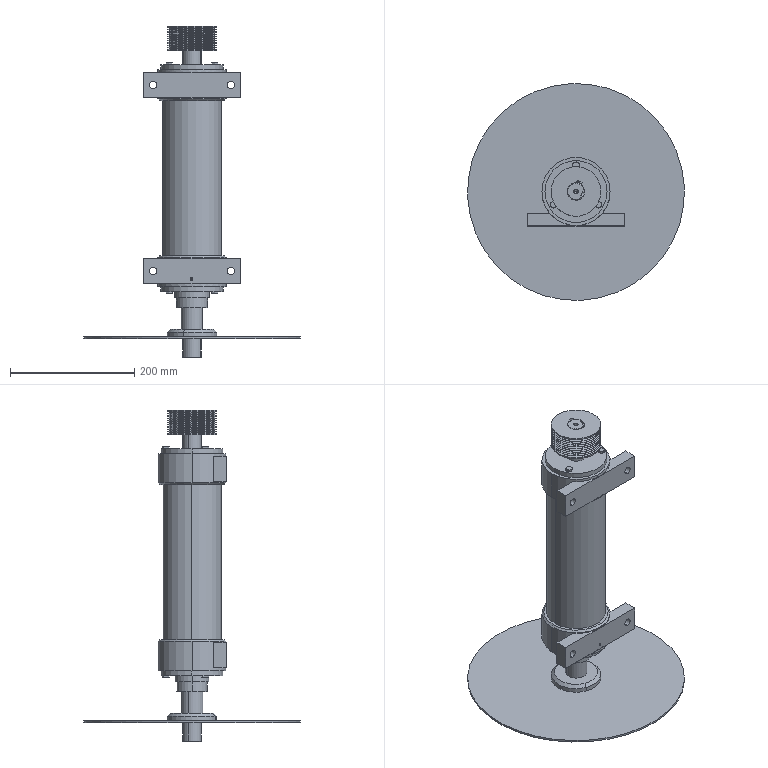Part | SolidWorks | features CompositeCurve 3 | 46 solids | 960 faces | box 350 x 350 x 535 mm | volume 3158794 mm3 | plane 279 | cylinder 276 | torus 140 | sphere 124 | cone 112 | spline 29 | commonest cylinder face diameters 51.65 x29 55.35 x29 44.4 x27 47.6 x27 80 x24 73.1 x20